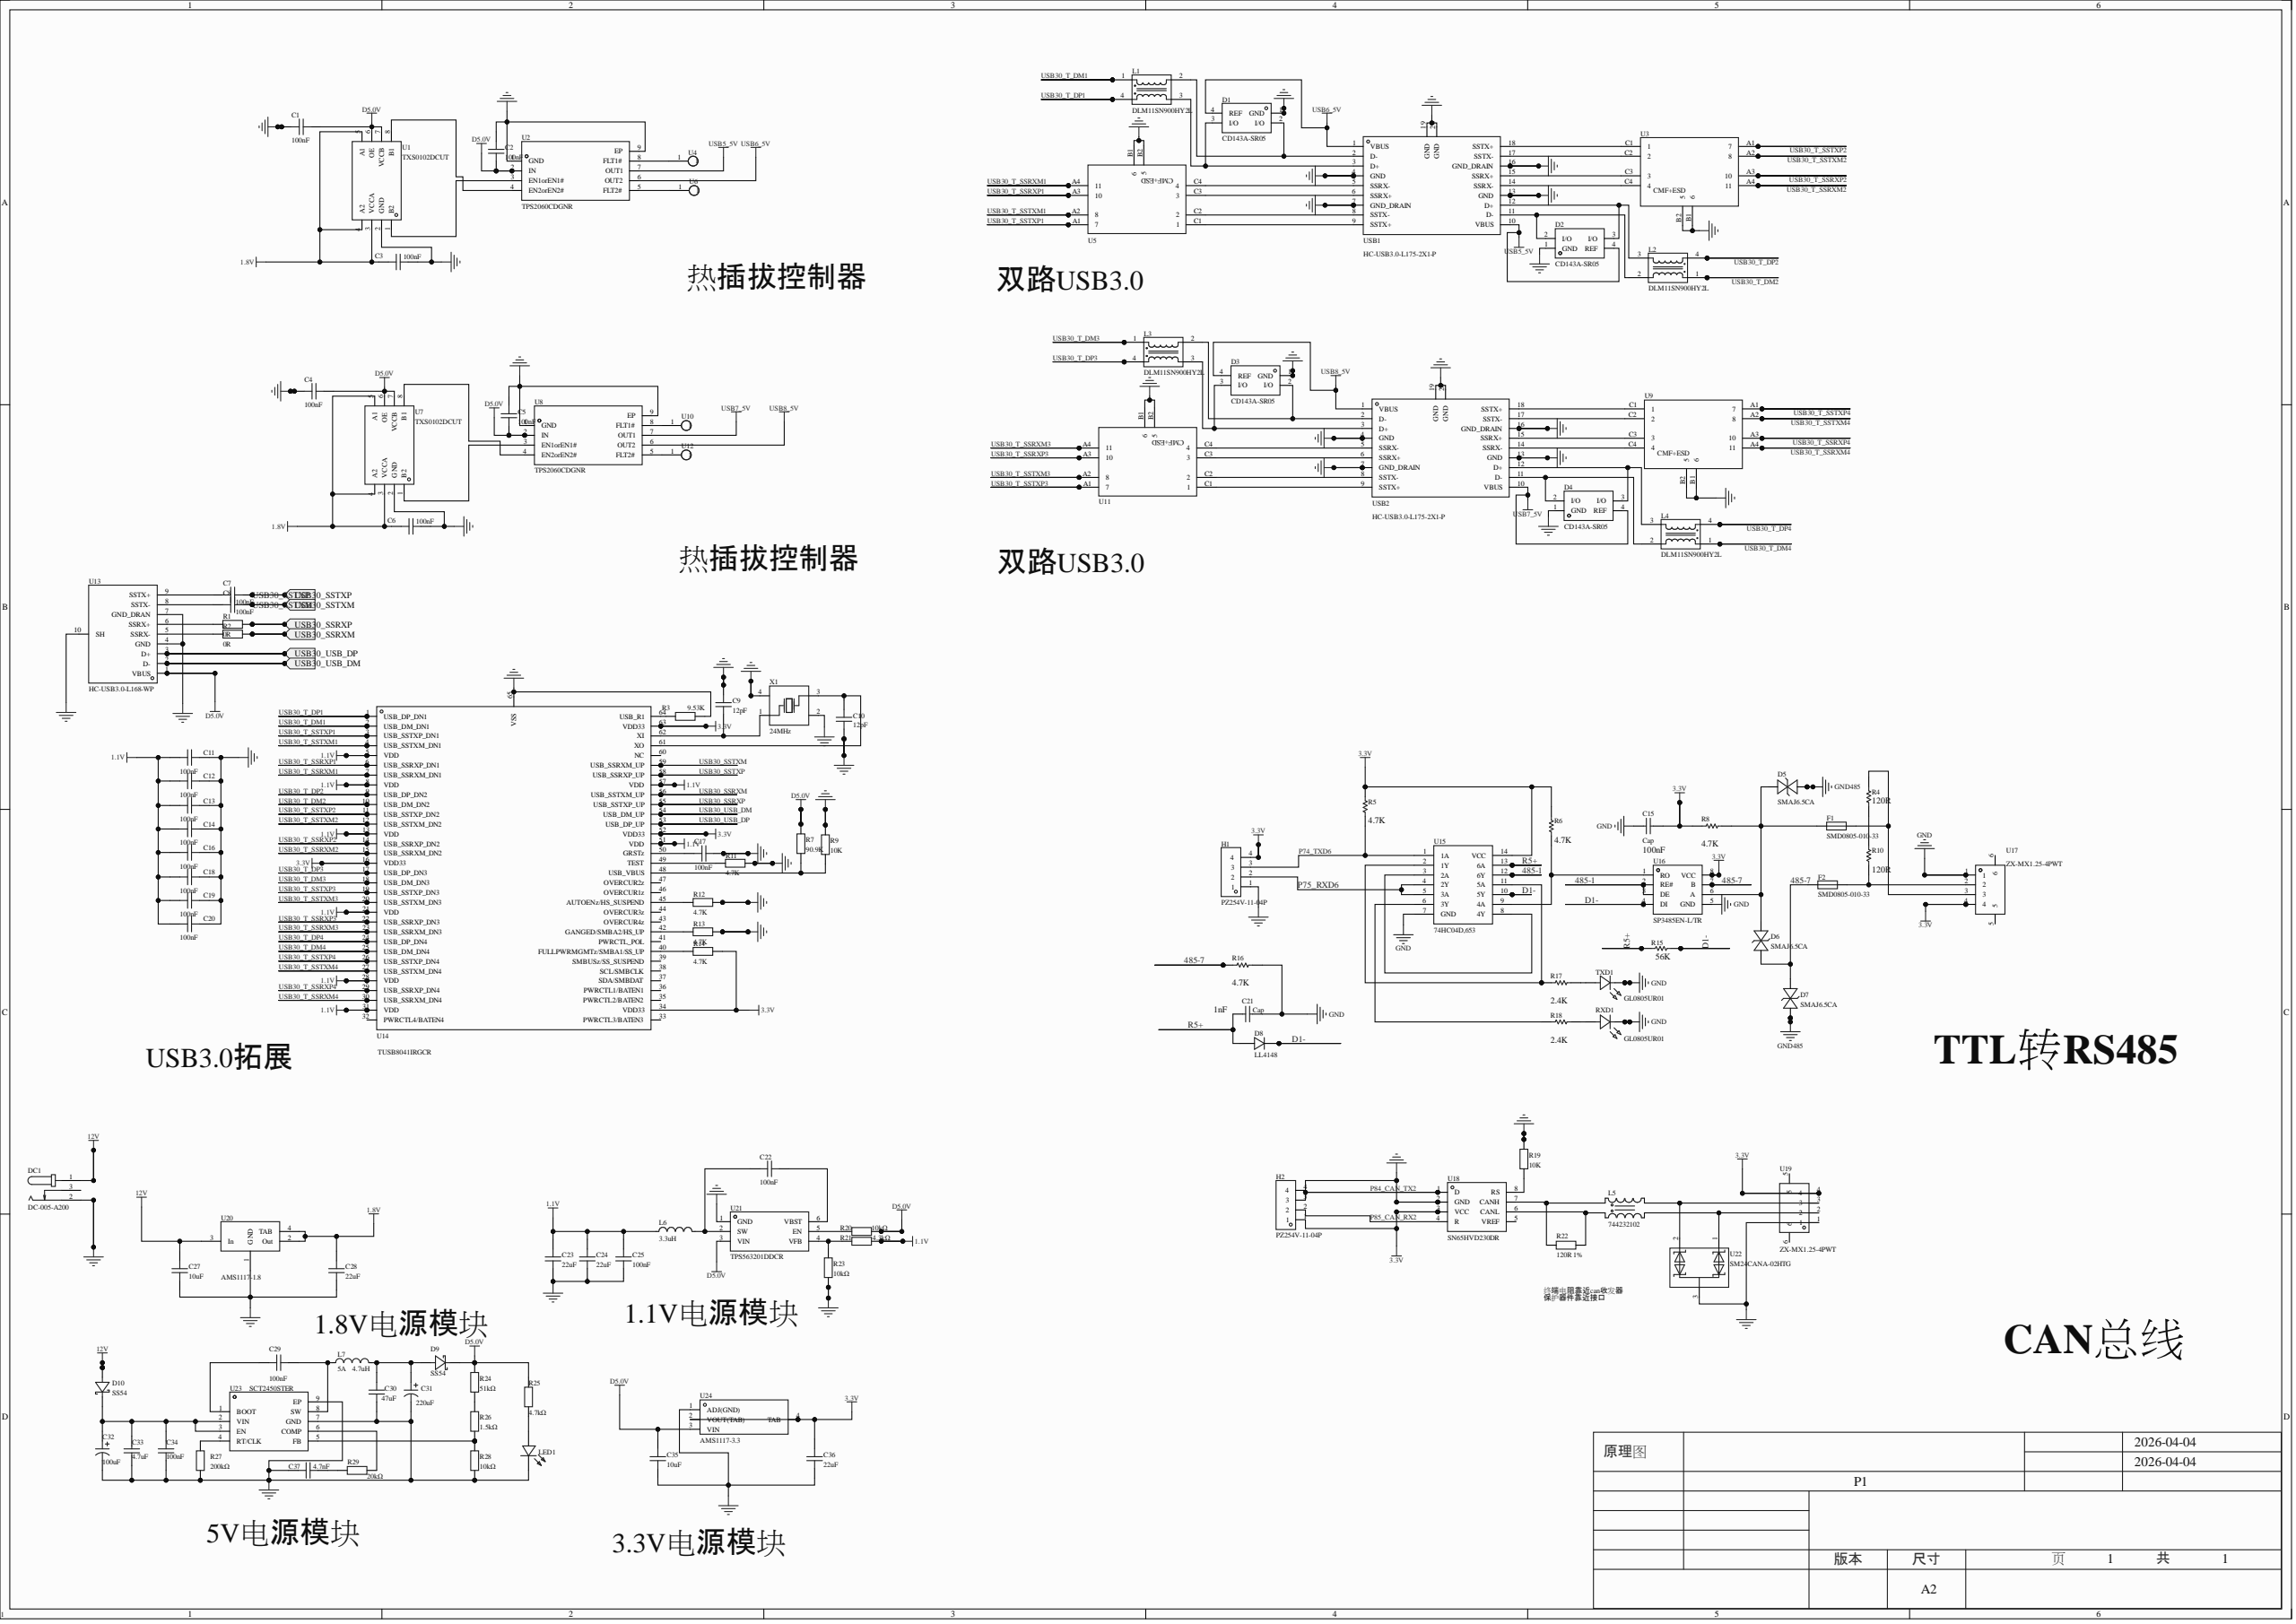Circuit board | Altium Designer | 117 parts | 119 nets
Bill of materials:
Comment,Description,Designator,Footprint,LibRef,Quantity
"100nF","","C1, C2, C3, C4, C5, C6, C7, C8, C11, C12, C13, C14, C16, C17, C18, C19, C20, C22, C25","C0402","CAP_0402, CAP_0603, CC0603KRX7R9BB104","19"
"12pF","","C9, C10","C0402","CAP_0603","2"
"Cap","Capacitor","C15, C21","C0402","Cap","2"
"22uF","","C23, C24, C28, C36","C0402","CGA0603X5R226M100JT, CAP_0603","4"
"10uF","","C27, C35","C0402","CAP_0603","2"
"100nF","","C29, C34","C0603","CL10B104KB8NNNC","2"
"47uF","","C30","C1206","GRM31CR61E476ME44L","1"
"220uF","","C31","CAP-SMD_BD6.3-L6.5-W6.5-LS7.2-FD","M2221M025C090RT","1"
"100uF","","C32","CAP-SMD_BD6.3-L6.5-W6.5-LS7.0-FD","SVZ1VM101E09E00RAXXX","1"
"4.7uF","","C33","C0603","CL31B475KBHNNNE","1"
"4.7nF","","C37","C0603","MT18B472K500CT","1"
"CD143A-SR05","","D1, D2, D3, D4","SOT-143_L2.9-W1.3-P1.92-LS2.3-BL","CD143A-SR05","4"
"SMAJ6.5CA","","D5, D6, D7","SMA-L4.3-W2.6-LS5.3-BI","SMAJ6.5CA_C19077527","3"
"LL4148","","D8","LL-34_L3.5-W1.5-RD","LL4148_C435829","1"
"SS54","","D9, D10","SMA_L4.4-W2.8-LS5.4-R-RD","SS54_C513478","2"
"DC-005-A200","","DC1","DC-IN-TH_DC-005-A200","DC-005-A200","1"
"SMD0805-010-33","","F1, F2","F0805","SMD0805-010-33","2"
"PZ254V-11-04P","","H1, H2","HDR-TH_4P-P2.54-V-M","PZ254V-11-04P","2"
"DLM11SN900HY2L","","L1, L2, L3, L4","FILTER-SMD_4P-L1.3-W1.0-TL_DLP11SN201HL2L","DLM11SN900HY2L","4"
"744232102","","L5","IND-SMD_4P-L3.2-W1.6","744232102","1"
"3.3uH","","L6","IND-SMD_L7.0-W6.6","FXL0630-3R3-M","1"
"4.7uH","","L7","IND-SMD_L7.0-W6.6","MWSA0624S-4R7MT","1"
"15-21VGC/TR8","","LED1","LED0603_GREEN","15-21VGC/TR8","1"
"0R","","R1, R2","R0402","Res_0603","2"
"9.53K","","R3","R0402","Res_0603","1"
"Res1","Resistor","R4, R5, R6, R8, R10, R15, R16, R17, R18","R0402","Res1","9"
"90.9K","","R7","R0402","Res_0603","1"
"10K","","R9, R19","R0402","Res_0603","2"
"4.7K","","R11, R12, R13, R14","R0402","Res_0603","4"
"10kΩ","","R20, R23, R28","R0402","0603WAF1002T5E, RC0603FR-074K7L","3"
"4.3kΩ","","R21","R0402","0603WAF4301T5E","1"
"120R 1%","","R22","R0402","Res_0603","1"
"51kΩ","","R24","R0402","RC0603FR-074K7L","1"
"4.7kΩ","","R25","R0402","RC0603FR-074K7L","1"
"1.5kΩ","","R26","R0402","RC0603FR-074K7L","1"
"200kΩ","","R27","R0402","RC0603FR-074K7L","1"
"20kΩ","","R29","R0402","RC0603FR-074K7L","1"
"GL0805UR01","","RXD1, TXD1","LED0805-R-RD_RED","GL0805UR01","2"
"TXS0102DCUT","","U1, U7","VSSOP-8_L2.3-W2.0-P0.50-LS3.1-BR","TXS0102DCUT","2"
"TPS2060CDGNR","","U2, U8","HVSSOP-8_L3.0-W3.0-P0.65-LS4.9-BL-EP-1","TPS2060CDGNR","2"
"","","U3, U5, U9, U11","PCMF2USB3S","PCMF2USB3S","4"
"","","U4, U6, U10, U12","tp点","tp点","4"
"HC-USB3.0-L168-WP","","U13","USB-TH_USB3.0-A","HC-USB3.0-L168-WP","1"
"TUSB8041IRGCR","","U14","QFN-64_L9.0-W9.0-P0.50-BL-EP7.2","TUSB8041IRGCR","1"
"74HC04D,653","","U15","SOIC-14_L8.7-W3.9-P1.27-LS6.0-BL","74HC04D,653","1"
"SP3485EN-L/TR","","U16","SOIC-8_L5.0-W4.0-P1.27-LS6.0-BL","SP3485EN-L/TR","1"
"ZX-MX1.25-4PWT","","U17, U19","CONN-SMD_4P-P1.25-MX1.25-4P-WT","ZX-MX1.25-4PWT","2"
"SN65HVD230DR","","U18","SOIC-8_L4.9-W3.9-P1.27-LS6.0-BL","SN65HVD230DR","1"
"AMS1117-1.8","","U20","SOT-223-4_L6.5-W3.5-P2.30-LS7.0-BR","AMS1117-1.8_C6185","1"
"TPS563201DDCR","","U21","SOT-23-6_L2.9-W1.6-P0.95-LS2.8-BR","TPS563201DDCR","1"
"SM24CANA-02HTG","","U22","SOT-23-3_L2.9-W1.3-P1.90-LS2.4-BR","SM24CANA-02HTG_C2936979","1"
"SCT2450STER","","U23","ESOP-8_L4.9-W3.9-P1.27-LS6.0-BL-EP","SCT2450STER","1"
"AMS1117-3.3","","U24","SOT-223-4_L6.5-W3.5-P2.30-LS7.0-BR","AMS1117-3.3_C347222","1"
"HC-USB3.0-L175-2X1-P","","USB1, USB2","USB-A-TH_H181-AF2R06-12ALCR","HC-USB3.0-L175-2X1-P","2"
"24MHz","","X1","CRYSTAL-SMD_4P-L3.2-W2.5-BL","X322524MOB4SI","1"
Netlist (Protel format):
[
C1
C0402
100nF



]
[
C2
C0402
100nF



]
[
C3
C0402
100nF



]
[
C4
C0402
100nF



]
[
C5
C0402
100nF



]
[
C6
C0402
100nF



]
[
C7
C0402
100nF



]
[
C8
C0402
100nF



]
[
C9
C0402
12pF



]
[
C10
C0402
12pF



]
[
C11
C0402
100nF



]
[
C12
C0402
100nF



]
[
C13
C0402
100nF



]
[
C14
C0402
100nF



]
[
C15
C0402
Cap



]
[
C16
C0402
100nF



]
[
C17
C0402
100nF



]
[
C18
C0402
100nF



]
[
C19
C0402
100nF



]
[
C20
C0402
100nF



]
[
C21
C0402
Cap



]
[
C22
C0402
100nF



]
[
C23
C0402
22uF



]
[
C24
C0402
22uF



]
[
C25
C0402
100nF



]
[
C27
C0402
10uF



]
[
C28
C0402
22uF



]
[
C29
C0603
100nF



]
[
C30
C1206
47uF



]
[
C31
CAP-SMD_BD6.3-L6.5-W6.5-LS7.2-FD
220uF



]
[
C32
CAP-SMD_BD6.3-L6.5-W6.5-LS7.0-FD
100uF



]
[
C33
C0603
4.7uF



]
[
C34
C0603
100nF



]
[
C35
C0402
10uF



]
[
C36
C0402
22uF



]
[
C37
C0603
4.7nF



]
[
D1
SOT-143_L2.9-W1.3-P1.92-LS2.3-BL
CD143A-SR05



]
[
D2
SOT-143_L2.9-W1.3-P1.92-LS2.3-BL
CD143A-SR05



]
[
D3
SOT-143_L2.9-W1.3-P1.92-LS2.3-BL
CD143A-SR05



]
[
D4
SOT-143_L2.9-W1.3-P1.92-LS2.3-BL
CD143A-SR05



]
[
D5
SMA-L4.3-W2.6-LS5.3-BI
SMAJ6.5CA



]
[
D6
SMA-L4.3-W2.6-LS5.3-BI
SMAJ6.5CA



]
[
D7
SMA-L4.3-W2.6-LS5.3-BI
SMAJ6.5CA



]
[
D8
LL-34_L3.5-W1.5-RD
LL4148



]
[
D9
SMA_L4.4-W2.8-LS5.4-R-RD
SS54



]
[
D10
SMA_L4.4-W2.8-LS5.4-R-RD
SS54



]
[
DC1
DC-IN-TH_DC-005-A200
DC-005-A200



]
[
F1
F0805
SMD0805-010-33



]
[
F2
F0805
SMD0805-010-33



]
[
H1
HDR-TH_4P-P2.54-V-M
PZ254V-11-04P



]
[
H2
HDR-TH_4P-P2.54-V-M
PZ254V-11-04P



]
[
L1
FILTER-SMD_4P-L1.3-W1.0-TL_DLP11SN201HL2L
DLM11SN900HY2L



]
[
L2
FILTER-SMD_4P-L1.3-W1.0-TL_DLP11SN201HL2L
DLM11SN900HY2L



]
[
L3
FILTER-SMD_4P-L1.3-W1.0-TL_DLP11SN201HL2L
DLM11SN900HY2L



]
[
L4
FILTER-SMD_4P-L1.3-W1.0-TL_DLP11SN201HL2L
DLM11SN900HY2L



]
[
L5
IND-SMD_4P-L3.2-W1.6
744232102



]
[
L6
IND-SMD_L7.0-W6.6
3.3uH



]
[
L7
IND-SMD_L7.0-W6.6
4.7uH



]
[
LED1
LED0603_GREEN
15-21VGC/TR8



]
[
R1
R0402
0R



]
[
R2
R0402
0R



]
[
R3
R0402
9.53K



]
[
R4
R0402
Res1



]
[
R5
R0402
Res1



]
[
R6
R0402
Res1



]
[
R7
R0402
90.9K



]
[
R8
R0402
Res1



]
[
R9
R0402
10K



]
[
R10
R0402
Res1



]
[
R11
R0402
4.7K



]
[
R12
R0402
4.7K



]
[
R13
R0402
4.7K



]
[
R14
R0402
4.7K



]
[
R15
R0402
Res1



]
[
R16
R0402
Res1



]
[
R17
R0402
Res1



]
[
R18
R0402
Res1



]
[
R19
R0402
10K



]
[
R20
R0402
10kΩ



]
[
R21
R0402
4.3kΩ



]
[
R22
R0402
120R 1%



]
[
R23
R0402
10kΩ



]
[
R24
R0402
51kΩ



]
[
R25
R0402
4.7kΩ



]
[
R26
R0402
1.5kΩ



]
[
R27
R0402
200kΩ



]
[
R28
R0402
10kΩ



]
[
R29
R0402
20kΩ



]
[
RXD1
LED0805-R-RD_RED
GL0805UR01



]
[
TXD1
LED0805-R-RD_RED
GL0805UR01



]
[
U1
VSSOP-8_L2.3-W2.0-P0.50-LS3.1-BR
TXS0102DCUT



]
[
U2
HVSSOP-8_L3.0-W3.0-P0.65-LS4.9-BL-EP-1
TPS2060CDGNR



]
[
U3
PCMF2USB3S




]
[
U4
tp点




]
[
U5
PCMF2USB3S




]
[
U6
tp点




]
[
U7
VSSOP-8_L2.3-W2.0-P0.50-LS3.1-BR
TXS0102DCUT



]
[
U8
HVSSOP-8_L3.0-W3.0-P0.65-LS4.9-BL-EP-1
TPS2060CDGNR



]
[
U9
PCMF2USB3S




]
[
U10
tp点




]
[
U11
PCMF2USB3S




]
[
U12
tp点




]
[
U13
USB-TH_USB3.0-A
HC-USB3.0-L168-WP



]
[
U14
QFN-64_L9.0-W9.0-P0.50-BL-EP7.2
TUSB8041IRGCR



]
[
U15
SOIC-14_L8.7-W3.9-P1.27-LS6.0-BL
74HC04D,653



]
[
U16
SOIC-8_L5.0-W4.0-P1.27-LS6.0-BL
SP3485EN-L/TR



]
[
U17
CONN-SMD_4P-P1.25-MX1.25-4P-WT
ZX-MX1.25-4PWT



]
[
U18
SOIC-8_L4.9-W3.9-P1.27-LS6.0-BL
SN65HVD230DR



]
[
U19
CONN-SMD_4P-P1.25-MX1.25-4P-WT
ZX-MX1.25-4PWT



]
[
U20
SOT-223-4_L6.5-W3.5-P2.30-LS7.0-BR
AMS1117-1.8



]
[
U21
SOT-23-6_L2.9-W1.6-P0.95-LS2.8-BR
TPS563201DDCR



]
[
U22
SOT-23-3_L2.9-W1.3-P1.90-LS2.4-BR
SM24CANA-02HTG



]
[
U23
ESOP-8_L4.9-W3.9-P1.27-LS6.0-BL-EP
SCT2450STER



]
[
U24
SOT-223-4_L6.5-W3.5-P2.30-LS7.0-BR
AMS1117-3.3



]
[
USB1
USB-A-TH_H181-AF2R06-12ALCR
HC-USB3.0-L175-2X1-P



]
[
USB2
USB-A-TH_H181-AF2R06-12ALCR
HC-USB3.0-L175-2X1-P



]
[
X1
CRYSTAL-SMD_4P-L3.2-W2.5-BL
24MHz



]
(
USB30_T_SSTXP4
U9-A1
U14-26
)
(
USB30_T_SSTXP3
U11-A1
U14-19
)
(
USB30_T_SSTXP2
U3-A1
U14-11
)
(
USB30_T_SSTXP1
U5-A1
U14-3
)
(
USB30_T_SSTXM4
U9-A2
U14-27
)
(
USB30_T_SSTXM3
U11-A2
U14-20
)
(
USB30_T_SSTXM2
U3-A2
U14-12
)
(
USB30_T_SSTXM1
U5-A2
U14-4
)
(
USB30_T_SSRXP4
U9-A3
U14-29
)
(
USB30_T_SSRXP3
U11-A3
U14-22
)
(
USB30_T_SSRXP2
U3-A3
U14-14
)
(
USB30_T_SSRXP1
U5-A3
U14-6
)
(
USB30_T_SSRXM4
U9-A4
U14-30
)
(
USB30_T_SSRXM3
U11-A4
U14-23
)
(
USB30_T_SSRXM2
U3-A4
U14-15
)
(
USB30_T_SSRXM1
U5-A4
U14-7
)
(
USB30_T_DP4
L4-4
U14-24
)
(
USB30_T_DP3
L3-4
U14-17
)
(
USB30_T_DP2
L2-4
U14-9
)
(
USB30_T_DP1
L1-4
U14-1
)
(
USB30_T_DM4
L4-1
U14-25
)
(
USB30_T_DM3
L3-1
U14-18
)
(
USB30_T_DM2
L2-1
U14-10
)
(
USB30_T_DM1
L1-1
U14-2
)
(
USB30_SSTXP
C7-2
U14-58
)
(
USB30_SSTXM
C8-2
U14-59
)
(
USB8_5V
D3-4
U8-6
USB2-1
)
(
USB7_5V
D4-4
U8-7
USB2-10
)
(
USB6_5V
D1-4
U2-6
USB1-1
)
(
USB5_5V
D2-4
U2-7
USB1-10
)
(
R5+
C21-2
D8-2
R15-2
U15-13
)
(
P85_CAN_RX2
H2-2
U18-4
)
(
P84_CAN_TX2
H2-3
U18-1
)
(
P75_RXD6
H1-2
U15-4
U15-5
)
(
P74_TXD6
H1-3
R5-1
U15-1
)
(
NetU15_3
U15-3
U15-8
)
(
NetU11_C4
U11-C4
USB2-5
)
(
NetU11_C3
U11-C3
USB2-6
)
(
NetU11_C2
U11-C2
USB2-8
)
(
NetU11_C1
U11-C1
USB2-9
)
(
NetU9_C4
U9-C4
USB2-14
)
(
NetU9_C3
U9-C3
USB2-15
)
(
NetU9_C2
U9-C2
USB2-17
)
(
NetU9_C1
U9-C1
USB2-18
)
(
NetU8_8
U8-8
U10-1
)
(
NetU8_5
U8-5
U12-1
)
(
NetU7_8
U7-8
U8-4
)
(
NetU7_1
U7-1
U8-3
)
(
NetU5_C4
U5-C4
USB1-5
)
(
NetU5_C3
U5-C3
USB1-6
)
(
NetU5_C2
U5-C2
USB1-8
)
(
NetU5_C1
U5-C1
USB1-9
)
(
NetU3_C4
U3-C4
USB1-14
)
(
NetU3_C3
U3-C3
USB1-15
)
(
NetU3_C2
U3-C2
USB1-17
)
(
NetU3_C1
U3-C1
USB1-18
)
(
NetU2_8
U2-8
U4-1
)
(
NetU2_5
U2-5
U6-1
)
(
NetU1_8
U1-8
U2-4
)
(
NetU1_1
U1-1
U2-3
)
(
NetR29_1
R29-1
U23-6
)
(
NetR27_2
R27-2
U23-4
)
(
NetR26_2
R26-2
R28-1
U23-5
)
(
NetR24_2
R24-2
R26-1
)
(
NetR21_1
R21-1
R23-1
U21-4
)
(
NetR20_1
R20-1
U21-5
)
(
NetR19_1
R19-1
U18-8
)
(
NetR18_2
R18-2
U15-6
)
(
NetR18_1
R18-1
RXD1-1
)
(
NetR17_2
R17-2
TXD1-1
)
(
NetR17_1
R17-1
U15-2
U15-11
)
(
NetR14_1
R14-1
U14-40
)
(
NetR13_1
R13-1
U14-42
)
(
NetR12_1
R12-1
U14-45
)
(
NetR11_1
R11-1
U14-49
)
(
NetR7_1
R7-1
R9-1
U14-48
)
(
NetR6_1
R6-1
U15-9
U16-1
)
(
NetR4_2
R4-2
R10-2
)
(
NetR3_1
R3-1
U14-64
)
(
NetR2_1
R2-1
U13-5
)
(
NetR1_1
R1-1
U13-6
)
(
NetLED1_1
LED1-1
R25-2
)
(
NetL5_4
L5-4
R22-2
U18-7
)
(
NetL5_3
L5-3
U19-3
U22-2
)
(
NetL5_2
L5-2
U19-2
U22-1
)
(
NetL5_1
L5-1
R22-1
U18-6
)
(
NetF2_2
F2-2
R10-1
U17-2
)
(
NetF1_2
F1-2
R4-1
U17-3
)
(
NetD5_1
D5-1
D6-2
F1-1
R8-1
U16-6
)
(
NetD4_3
D4-3
L4-3
USB2-12
)
(
NetD4_2
D4-2
L4-2
USB2-11
)
(
NetD3_3
D3-3
L3-3
USB2-3
)
(
NetD3_2
D3-2
L3-2
USB2-2
)
(
NetD2_3
D2-3
L2-3
USB1-12
)
(
NetD2_2
D2-2
L2-2
USB1-11
)
(
NetD1_3
D1-3
L1-3
USB1-3
)
(
NetD1_2
D1-2
L1-2
USB1-2
)
(
NetC37_1
C37-1
R29-2
)
(
NetC32_1
C32-1
C33-2
C34-2
D10-2
U23-2
U23-3
)
(
NetC30_2
C30-2
C31-1
D9-1
L7-2
)
(
NetC29_2
C29-2
U23-1
)
(
NetC29_1
C29-1
L7-1
U23-8
)
(
NetC22_2
C22-2
U21-6
)
(
NetC22_1
C22-1
L6-2
U21-2
)
(
NetC17_1
C17-1
U14-50
)
(
NetC10_2
C10-2
U14-61
X1-3
)
(
NetC9_2
C9-2
U14-62
X1-1
)
(
NetC8_1
C8-1
U13-8
)
(
NetC7_1
C7-1
U13-9
)
(
GND485
D5-2
D7-1
)
(
GND
C1-1
C2-2
C3-2
C4-1
C5-2
C6-2
C9-1
C10-1
C11-1
C12-1
C13-1
C14-1
C15-2
C16-1
C17-2
C18-1
C19-1
C20-1
C21-1
C23-1
C24-1
C25-1
C27-1
C28-1
C30-1
C31-2
C32-2
C33-1
C34-1
C35-1
C36-1
C37-2
D1-1
D2-1
D3-1
D4-1
DC1-2
H1-1
H2-4
LED1-2
R3-2
R9-2
R11-2
R12-2
R13-2
R16-1
R19-2
R23-2
R27-1
R28-2
RXD1-2
TXD1-2
U1-2
U2-1
U2-9
U3-B1
U3-B2
U5-B1
U5-B2
U7-2
U8-1
U8-9
U9-B1
U9-B2
U11-B1
U11-B2
U13-4
U13-7
U13-10
U14-65
U15-7
U16-5
U17-1
U18-2
U19-1
U20-1
U21-1
U22-3
U23-7
U23-9
U24-1
USB1-4
USB1-7
USB1-13
USB1-16
USB1-19
USB1-20
USB2-4
USB2-7
USB2-13
USB2-16
USB2-19
USB2-20
X1-2
X1-4
)
(
D5.0V
C1-2
C2-1
C4-2
C5-1
C35-2
D9-2
R7-2
R20-2
R24-1
R25-1
U1-6
U1-7
U2-2
U7-6
U7-7
U8-2
U13-1
U21-3
U24-3
)
(
D1-
D8-1
R15-1
U15-10
U16-4
)
(
485-7
D6-1
D7-2
F2-1
R16-2
U16-7
)
(
485-1
U15-12
U16-2
U16-3
)
(
12V
C27-2
D10-1
DC1-1
U20-3
)
(
3.3V
C15-1
C36-2
H1-4
H2-1
R5-2
R6-2
R8-2
R14-2
U14-16
U14-34
U14-52
U14-63
U15-14
U16-8
U17-4
U18-3
U19-4
U24-2
U24-4
)
(
1.8V
C3-1
C6-1
C28-2
U1-3
U1-4
U1-5
U7-3
U7-4
U7-5
U20-2
U20-4
)
(
1.1V
C11-2
C12-2
C13-2
C14-2
C16-2
C18-2
C19-2
C20-2
C23-2
C24-2
C25-2
L6-1
R21-2
U14-5
U14-8
U14-13
U14-21
U14-28
U14-31
U14-51
U14-57
)